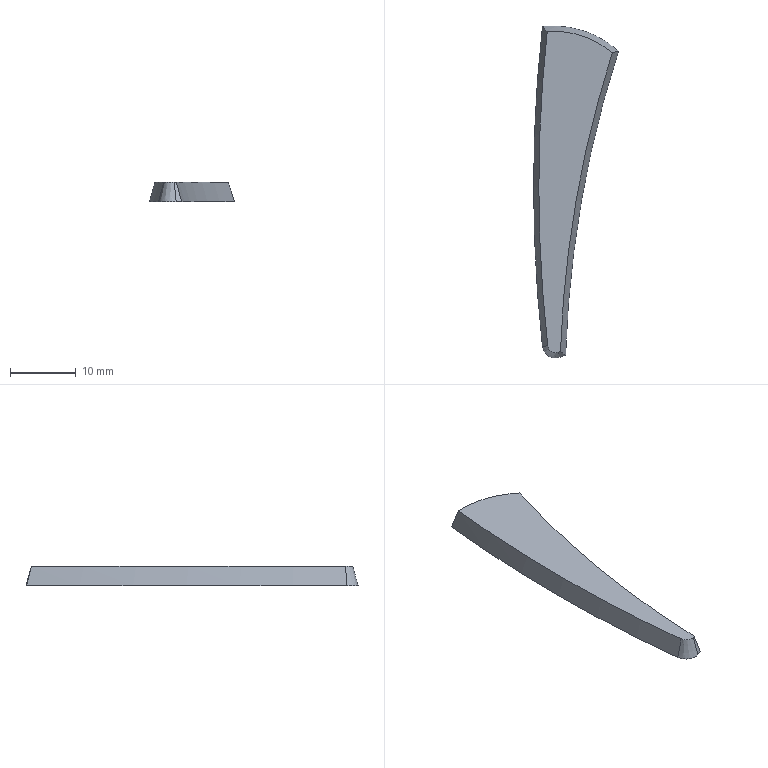Part | STEP file | Twistgrip Indicator LensMirror 3 speed | 1 solid | 7 faces | box 12.929 x 50.6 x 3 mm | volume 990.218 mm3 | cone 4 | plane 3
STEP:
#1=CARTESIAN_POINT('',(0.,0.,0.));
#2=DIRECTION('',(0.,0.,1.));
#3=DIRECTION('',(1.,0.,0.));
#4=AXIS2_PLACEMENT_3D('',#1,#2,#3);
#5=CARTESIAN_POINT('',(-17.743,-15.241,-3.));
#6=VERTEX_POINT('',#5);
#7=CARTESIAN_POINT('',(-18.67,-15.499,0.));
#8=VERTEX_POINT('',#7);
#9=CARTESIAN_POINT('',(-17.743,-15.241,-3.));
#10=CARTESIAN_POINT('',(-18.051,-15.323,-1.999));
#11=CARTESIAN_POINT('',(-18.36,-15.409,-0.9995));
#12=CARTESIAN_POINT('',(-18.67,-15.499,0.));
#13=B_SPLINE_CURVE_WITH_KNOTS('',3,(#9,#10,#11,#12),.UNSPECIFIED.,.F.,.F.,(4,4),(0.,0.003151),.PIECEWISE_BEZIER_KNOTS.);
#14=CARTESIAN_POINT('',(142.328,-66.926,0.));
#15=DIRECTION('',(0.,0.,1.));
#16=DIRECTION('',(1.,0.,0.));
#17=AXIS2_PLACEMENT_3D('',#14,#15,#16);
#18=CONICAL_SURFACE('',#17,169.012,0.2618);
#19=CARTESIAN_POINT('',(2.829,-3.));
#20=CARTESIAN_POINT('',(2.829,-2.955));
#21=CARTESIAN_POINT('',(2.829,-2.864));
#22=CARTESIAN_POINT('',(2.83,-2.727));
#23=CARTESIAN_POINT('',(2.83,-2.591));
#24=CARTESIAN_POINT('',(2.83,-2.454));
#25=CARTESIAN_POINT('',(2.83,-2.318));
#26=CARTESIAN_POINT('',(2.83,-2.182));
#27=CARTESIAN_POINT('',(2.83,-2.045));
#28=CARTESIAN_POINT('',(2.83,-1.909));
#29=CARTESIAN_POINT('',(2.831,-1.772));
#30=CARTESIAN_POINT('',(2.831,-1.636));
#31=CARTESIAN_POINT('',(2.831,-1.5));
#32=CARTESIAN_POINT('',(2.831,-1.363));
#33=CARTESIAN_POINT('',(2.831,-1.227));
#34=CARTESIAN_POINT('',(2.831,-1.091));
#35=CARTESIAN_POINT('',(2.831,-0.9542));
#36=CARTESIAN_POINT('',(2.832,-0.8179));
#37=CARTESIAN_POINT('',(2.832,-0.6815));
#38=CARTESIAN_POINT('',(2.832,-0.5452));
#39=CARTESIAN_POINT('',(2.832,-0.4089));
#40=CARTESIAN_POINT('',(2.832,-0.2726));
#41=CARTESIAN_POINT('',(2.832,-0.1363));
#42=CARTESIAN_POINT('',(2.832,-0.04543));
#43=CARTESIAN_POINT('',(2.832,0.));
#44=B_SPLINE_CURVE_WITH_KNOTS('',3,(#19,#20,#21,#22,#23,#24,#25,#26,#27,#28,#29,#30,#31,#32,#33,#34,#35,#36,#37,#38,#39,#40,#41,#42,#43),.UNSPECIFIED.,.F.,.F.,(4,1,1,1,1,1,1,1,1,1,1,1,1,1,1,1,1,1,1,1,1,1,4),(0.,0.0001432,0.0002864,0.0004296,0.0005728,0.000716,0.0008592,0.001002,0.001146,0.001289,0.001432,0.001575,0.001718,0.001862,0.002005,0.002148,0.002291,0.002435,0.002578,0.002721,0.002864,0.003007,0.003151),.QUASI_UNIFORM_KNOTS.);
#45=(GEOMETRIC_REPRESENTATION_CONTEXT(2)PARAMETRIC_REPRESENTATION_CONTEXT()REPRESENTATION_CONTEXT('',''));
#46=DEFINITIONAL_REPRESENTATION('',(#44),#45);
#47=PCURVE('',#18,#46);
#48=CARTESIAN_POINT('',(-27.685,-26.228,0.));
#49=DIRECTION('',(0.,0.,-1.));
#50=DIRECTION('',(1.,0.,0.));
#51=AXIS2_PLACEMENT_3D('',#48,#49,#50);
#52=CONICAL_SURFACE('',#51,14.014,0.2618);
#53=CARTESIAN_POINT('',(5.448,3.));
#54=CARTESIAN_POINT('',(5.447,2.955));
#55=CARTESIAN_POINT('',(5.446,2.864));
#56=CARTESIAN_POINT('',(5.445,2.727));
#57=CARTESIAN_POINT('',(5.443,2.591));
#58=CARTESIAN_POINT('',(5.441,2.454));
#59=CARTESIAN_POINT('',(5.44,2.318));
#60=CARTESIAN_POINT('',(5.438,2.182));
#61=CARTESIAN_POINT('',(5.437,2.045));
#62=CARTESIAN_POINT('',(5.435,1.909));
#63=CARTESIAN_POINT('',(5.433,1.772));
#64=CARTESIAN_POINT('',(5.432,1.636));
#65=CARTESIAN_POINT('',(5.43,1.5));
#66=CARTESIAN_POINT('',(5.428,1.363));
#67=CARTESIAN_POINT('',(5.427,1.227));
#68=CARTESIAN_POINT('',(5.425,1.091));
#69=CARTESIAN_POINT('',(5.423,0.9542));
#70=CARTESIAN_POINT('',(5.422,0.8179));
#71=CARTESIAN_POINT('',(5.42,0.6815));
#72=CARTESIAN_POINT('',(5.418,0.5452));
#73=CARTESIAN_POINT('',(5.416,0.4089));
#74=CARTESIAN_POINT('',(5.415,0.2726));
#75=CARTESIAN_POINT('',(5.413,0.1363));
#76=CARTESIAN_POINT('',(5.412,0.04543));
#77=CARTESIAN_POINT('',(5.411,0.));
#78=B_SPLINE_CURVE_WITH_KNOTS('',3,(#53,#54,#55,#56,#57,#58,#59,#60,#61,#62,#63,#64,#65,#66,#67,#68,#69,#70,#71,#72,#73,#74,#75,#76,#77),.UNSPECIFIED.,.F.,.F.,(4,1,1,1,1,1,1,1,1,1,1,1,1,1,1,1,1,1,1,1,1,1,4),(0.,0.0001432,0.0002864,0.0004296,0.0005728,0.000716,0.0008592,0.001002,0.001146,0.001289,0.001432,0.001575,0.001718,0.001862,0.002005,0.002148,0.002291,0.002435,0.002578,0.002721,0.002864,0.003007,0.003151),.QUASI_UNIFORM_KNOTS.);
#79=(GEOMETRIC_REPRESENTATION_CONTEXT(2)PARAMETRIC_REPRESENTATION_CONTEXT()REPRESENTATION_CONTEXT('',''));
#80=DEFINITIONAL_REPRESENTATION('',(#78),#79);
#81=PCURVE('',#52,#80);
#82=SURFACE_CURVE('',#13,(#47,#81),.PCURVE_S1.);
#83=EDGE_CURVE('',#6,#8,#82,.T.);
#84=ORIENTED_EDGE('',*,*,#83,.F.);
#85=CARTESIAN_POINT('',(-25.795,-61.568,-3.));
#86=VERTEX_POINT('',#85);
#87=CARTESIAN_POINT('',(142.328,-66.926,-3.));
#88=DIRECTION('',(0.,0.,-1.));
#89=DIRECTION('',(1.,0.,0.));
#90=AXIS2_PLACEMENT_3D('',#87,#88,#89);
#91=CIRCLE('',#90,168.208);
#92=CARTESIAN_POINT('',(6.283,-3.));
#93=DIRECTION('',(-1.,0.));
#94=VECTOR('',#93,1.);
#95=LINE('',#92,#94);
#96=(GEOMETRIC_REPRESENTATION_CONTEXT(2)PARAMETRIC_REPRESENTATION_CONTEXT()REPRESENTATION_CONTEXT('',''));
#97=DEFINITIONAL_REPRESENTATION('',(#95),#96);
#98=PCURVE('',#18,#97);
#99=CARTESIAN_POINT('',(142.328,-66.926,-3.));
#100=DIRECTION('',(0.,0.,-1.));
#101=DIRECTION('',(1.,0.,0.));
#102=AXIS2_PLACEMENT_3D('',#99,#100,#101);
#103=PLANE('',#102);
#104=CARTESIAN_POINT('',(0.,0.));
#105=DIRECTION('',(1.,0.));
#106=AXIS2_PLACEMENT_2D('',#104,#105);
#107=CIRCLE('',#106,168.208);
#108=(GEOMETRIC_REPRESENTATION_CONTEXT(2)PARAMETRIC_REPRESENTATION_CONTEXT()REPRESENTATION_CONTEXT('',''));
#109=DEFINITIONAL_REPRESENTATION('',(#107),#108);
#110=PCURVE('',#103,#109);
#111=SURFACE_CURVE('',#91,(#98,#110),.PCURVE_S1.);
#112=EDGE_CURVE('',#86,#6,#111,.T.);
#113=ORIENTED_EDGE('',*,*,#112,.F.);
#114=CARTESIAN_POINT('',(-26.58,-61.005,0.));
#115=VERTEX_POINT('',#114);
#116=CARTESIAN_POINT('',(-25.795,-61.568,-3.));
#117=CARTESIAN_POINT('',(-26.057,-61.381,-2.));
#118=CARTESIAN_POINT('',(-26.319,-61.193,-1.));
#119=CARTESIAN_POINT('',(-26.58,-61.005,0.));
#120=B_SPLINE_CURVE_WITH_KNOTS('',3,(#116,#117,#118,#119),.UNSPECIFIED.,.F.,.F.,(4,4),(0.,0.003152),.PIECEWISE_BEZIER_KNOTS.);
#121=CARTESIAN_POINT('',(3.11,-3.));
#122=CARTESIAN_POINT('',(3.11,-2.955));
#123=CARTESIAN_POINT('',(3.11,-2.864));
#124=CARTESIAN_POINT('',(3.109,-2.727));
#125=CARTESIAN_POINT('',(3.109,-2.591));
#126=CARTESIAN_POINT('',(3.109,-2.455));
#127=CARTESIAN_POINT('',(3.109,-2.318));
#128=CARTESIAN_POINT('',(3.109,-2.182));
#129=CARTESIAN_POINT('',(3.109,-2.045));
#130=CARTESIAN_POINT('',(3.109,-1.909));
#131=CARTESIAN_POINT('',(3.108,-1.773));
#132=CARTESIAN_POINT('',(3.108,-1.636));
#133=CARTESIAN_POINT('',(3.108,-1.5));
#134=CARTESIAN_POINT('',(3.108,-1.364));
#135=CARTESIAN_POINT('',(3.108,-1.227));
#136=CARTESIAN_POINT('',(3.108,-1.091));
#137=CARTESIAN_POINT('',(3.108,-0.9546));
#138=CARTESIAN_POINT('',(3.107,-0.8182));
#139=CARTESIAN_POINT('',(3.107,-0.6818));
#140=CARTESIAN_POINT('',(3.107,-0.5455));
#141=CARTESIAN_POINT('',(3.107,-0.4091));
#142=CARTESIAN_POINT('',(3.107,-0.2727));
#143=CARTESIAN_POINT('',(3.107,-0.1364));
#144=CARTESIAN_POINT('',(3.107,-0.04546));
#145=CARTESIAN_POINT('',(3.107,0.));
#146=B_SPLINE_CURVE_WITH_KNOTS('',3,(#121,#122,#123,#124,#125,#126,#127,#128,#129,#130,#131,#132,#133,#134,#135,#136,#137,#138,#139,#140,#141,#142,#143,#144,#145),.UNSPECIFIED.,.F.,.F.,(4,1,1,1,1,1,1,1,1,1,1,1,1,1,1,1,1,1,1,1,1,1,4),(0.,0.0001433,0.0002865,0.0004298,0.0005731,0.0007163,0.0008596,0.001003,0.001146,0.001289,0.001433,0.001576,0.001719,0.001862,0.002006,0.002149,0.002292,0.002435,0.002579,0.002722,0.002865,0.003009,0.003152),.QUASI_UNIFORM_KNOTS.);
#147=(GEOMETRIC_REPRESENTATION_CONTEXT(2)PARAMETRIC_REPRESENTATION_CONTEXT()REPRESENTATION_CONTEXT('',''));
#148=DEFINITIONAL_REPRESENTATION('',(#146),#147);
#149=PCURVE('',#18,#148);
#150=CARTESIAN_POINT('',(-26.909,-61.129,0.));
#151=DIRECTION('',(0.3409,-0.9038,0.2588));
#152=DIRECTION('',(0.9357,0.3529,0.));
#153=AXIS2_PLACEMENT_3D('',#150,#151,#152);
#154=PLANE('',#153);
#155=CARTESIAN_POINT('',(0.8877,-3.106));
#156=CARTESIAN_POINT('',(0.7086,-2.071));
#157=CARTESIAN_POINT('',(0.5298,-1.035));
#158=CARTESIAN_POINT('',(0.3514,0.));
#159=B_SPLINE_CURVE_WITH_KNOTS('',3,(#155,#156,#157,#158),.UNSPECIFIED.,.F.,.F.,(4,4),(0.,0.003152),.PIECEWISE_BEZIER_KNOTS.);
#160=(GEOMETRIC_REPRESENTATION_CONTEXT(2)PARAMETRIC_REPRESENTATION_CONTEXT()REPRESENTATION_CONTEXT('',''));
#161=DEFINITIONAL_REPRESENTATION('',(#159),#160);
#162=PCURVE('',#154,#161);
#163=SURFACE_CURVE('',#120,(#149,#162),.PCURVE_S1.);
#164=EDGE_CURVE('',#86,#115,#163,.T.);
#165=ORIENTED_EDGE('',*,*,#164,.T.);
#166=CARTESIAN_POINT('',(142.328,-66.926,0.));
#167=DIRECTION('',(0.,0.,-1.));
#168=DIRECTION('',(1.,0.,0.));
#169=AXIS2_PLACEMENT_3D('',#166,#167,#168);
#170=CIRCLE('',#169,169.012);
#171=CARTESIAN_POINT('',(6.283,0.));
#172=DIRECTION('',(-1.,0.));
#173=VECTOR('',#172,1.);
#174=LINE('',#171,#173);
#175=(GEOMETRIC_REPRESENTATION_CONTEXT(2)PARAMETRIC_REPRESENTATION_CONTEXT()REPRESENTATION_CONTEXT('',''));
#176=DEFINITIONAL_REPRESENTATION('',(#174),#175);
#177=PCURVE('',#18,#176);
#178=CARTESIAN_POINT('',(142.328,-66.926,0.));
#179=DIRECTION('',(0.,0.,-1.));
#180=DIRECTION('',(1.,0.,0.));
#181=AXIS2_PLACEMENT_3D('',#178,#179,#180);
#182=PLANE('',#181);
#183=CARTESIAN_POINT('',(0.,0.));
#184=DIRECTION('',(1.,0.));
#185=AXIS2_PLACEMENT_2D('',#183,#184);
#186=CIRCLE('',#185,169.012);
#187=(GEOMETRIC_REPRESENTATION_CONTEXT(2)PARAMETRIC_REPRESENTATION_CONTEXT()REPRESENTATION_CONTEXT('',''));
#188=DEFINITIONAL_REPRESENTATION('',(#186),#187);
#189=PCURVE('',#182,#188);
#190=SURFACE_CURVE('',#170,(#177,#189),.PCURVE_S1.);
#191=EDGE_CURVE('',#115,#8,#190,.T.);
#192=ORIENTED_EDGE('',*,*,#191,.T.);
#193=EDGE_LOOP('',(#84,#113,#165,#192));
#194=FACE_BOUND('',#193,.F.);
#195=ADVANCED_FACE('',(#194),#18,.F.);
#196=CARTESIAN_POINT('',(-28.597,-12.244,0.));
#197=VERTEX_POINT('',#196);
#198=CARTESIAN_POINT('',(-27.685,-26.228,0.));
#199=DIRECTION('',(0.,0.,1.));
#200=DIRECTION('',(1.,0.,0.));
#201=AXIS2_PLACEMENT_3D('',#198,#199,#200);
#202=CIRCLE('',#201,14.014);
#203=CARTESIAN_POINT('',(6.283,0.));
#204=DIRECTION('',(-1.,0.));
#205=VECTOR('',#204,1.);
#206=LINE('',#203,#205);
#207=(GEOMETRIC_REPRESENTATION_CONTEXT(2)PARAMETRIC_REPRESENTATION_CONTEXT()REPRESENTATION_CONTEXT('',''));
#208=DEFINITIONAL_REPRESENTATION('',(#206),#207);
#209=PCURVE('',#52,#208);
#210=CARTESIAN_POINT('',(-155.999,-40.698));
#211=CARTESIAN_POINT('',(-155.999,-64.971));
#212=CARTESIAN_POINT('',(-177.02,-52.835));
#213=CARTESIAN_POINT('',(-198.041,-40.698));
#214=CARTESIAN_POINT('',(-177.02,-28.561));
#215=CARTESIAN_POINT('',(-155.999,-16.425));
#216=CARTESIAN_POINT('',(-155.999,-40.698));
#217=(BOUNDED_CURVE()B_SPLINE_CURVE(2,(#210,#211,#212,#213,#214,#215,#216),.UNSPECIFIED.,.T.,.F.)B_SPLINE_CURVE_WITH_KNOTS((1,2,2,2,2,1),(-2.094,0.,2.094,4.189,6.283,8.378),.UNSPECIFIED.)CURVE()GEOMETRIC_REPRESENTATION_ITEM()RATIONAL_B_SPLINE_CURVE((1.,0.5,1.,0.5,1.,0.5,1.))REPRESENTATION_ITEM(''));
#218=(GEOMETRIC_REPRESENTATION_CONTEXT(2)PARAMETRIC_REPRESENTATION_CONTEXT()REPRESENTATION_CONTEXT('',''));
#219=DEFINITIONAL_REPRESENTATION('',(#217),#218);
#220=PCURVE('',#182,#219);
#221=SURFACE_CURVE('',#202,(#209,#220),.PCURVE_S1.);
#222=EDGE_CURVE('',#8,#197,#221,.T.);
#223=ORIENTED_EDGE('',*,*,#222,.F.);
#224=ORIENTED_EDGE('',*,*,#83,.F.);
#225=CARTESIAN_POINT('',(-29.325,-11.501,-3.));
#226=VERTEX_POINT('',#225);
#227=CARTESIAN_POINT('',(-27.685,-26.228,-3.));
#228=DIRECTION('',(0.,0.,1.));
#229=DIRECTION('',(1.,0.,0.));
#230=AXIS2_PLACEMENT_3D('',#227,#228,#229);
#231=CIRCLE('',#230,14.818);
#232=CARTESIAN_POINT('',(6.283,3.));
#233=DIRECTION('',(-1.,0.));
#234=VECTOR('',#233,1.);
#235=LINE('',#232,#234);
#236=(GEOMETRIC_REPRESENTATION_CONTEXT(2)PARAMETRIC_REPRESENTATION_CONTEXT()REPRESENTATION_CONTEXT('',''));
#237=DEFINITIONAL_REPRESENTATION('',(#235),#236);
#238=PCURVE('',#52,#237);
#239=CARTESIAN_POINT('',(-155.195,-40.698));
#240=CARTESIAN_POINT('',(-155.195,-66.364));
#241=CARTESIAN_POINT('',(-177.422,-53.531));
#242=CARTESIAN_POINT('',(-199.649,-40.698));
#243=CARTESIAN_POINT('',(-177.422,-27.865));
#244=CARTESIAN_POINT('',(-155.195,-15.032));
#245=CARTESIAN_POINT('',(-155.195,-40.698));
#246=(BOUNDED_CURVE()B_SPLINE_CURVE(2,(#239,#240,#241,#242,#243,#244,#245),.UNSPECIFIED.,.T.,.F.)B_SPLINE_CURVE_WITH_KNOTS((1,2,2,2,2,1),(-2.094,0.,2.094,4.189,6.283,8.378),.UNSPECIFIED.)CURVE()GEOMETRIC_REPRESENTATION_ITEM()RATIONAL_B_SPLINE_CURVE((1.,0.5,1.,0.5,1.,0.5,1.))REPRESENTATION_ITEM(''));
#247=(GEOMETRIC_REPRESENTATION_CONTEXT(2)PARAMETRIC_REPRESENTATION_CONTEXT()REPRESENTATION_CONTEXT('',''));
#248=DEFINITIONAL_REPRESENTATION('',(#246),#247);
#249=PCURVE('',#103,#248);
#250=SURFACE_CURVE('',#231,(#238,#249),.PCURVE_S1.);
#251=EDGE_CURVE('',#6,#226,#250,.T.);
#252=ORIENTED_EDGE('',*,*,#251,.T.);
#253=CARTESIAN_POINT('',(-29.325,-11.501,-3.));
#254=CARTESIAN_POINT('',(-29.082,-11.744,-1.999));
#255=CARTESIAN_POINT('',(-28.839,-11.991,-0.9989));
#256=CARTESIAN_POINT('',(-28.597,-12.244,0.));
#257=B_SPLINE_CURVE_WITH_KNOTS('',3,(#253,#254,#255,#256),.UNSPECIFIED.,.F.,.F.,(4,4),(0.,0.003175),.PIECEWISE_BEZIER_KNOTS.);
#258=CARTESIAN_POINT('',(4.602,3.));
#259=CARTESIAN_POINT('',(4.602,2.954));
#260=CARTESIAN_POINT('',(4.603,2.863));
#261=CARTESIAN_POINT('',(4.605,2.727));
#262=CARTESIAN_POINT('',(4.607,2.591));
#263=CARTESIAN_POINT('',(4.609,2.454));
#264=CARTESIAN_POINT('',(4.612,2.318));
#265=CARTESIAN_POINT('',(4.614,2.181));
#266=CARTESIAN_POINT('',(4.616,2.045));
#267=CARTESIAN_POINT('',(4.618,1.908));
#268=CARTESIAN_POINT('',(4.62,1.772));
#269=CARTESIAN_POINT('',(4.622,1.636));
#270=CARTESIAN_POINT('',(4.624,1.499));
#271=CARTESIAN_POINT('',(4.626,1.363));
#272=CARTESIAN_POINT('',(4.628,1.226));
#273=CARTESIAN_POINT('',(4.63,1.09));
#274=CARTESIAN_POINT('',(4.632,0.9538));
#275=CARTESIAN_POINT('',(4.634,0.8175));
#276=CARTESIAN_POINT('',(4.636,0.6812));
#277=CARTESIAN_POINT('',(4.639,0.545));
#278=CARTESIAN_POINT('',(4.641,0.4087));
#279=CARTESIAN_POINT('',(4.643,0.2725));
#280=CARTESIAN_POINT('',(4.645,0.1362));
#281=CARTESIAN_POINT('',(4.647,0.0454));
#282=CARTESIAN_POINT('',(4.647,0.));
#283=B_SPLINE_CURVE_WITH_KNOTS('',3,(#258,#259,#260,#261,#262,#263,#264,#265,#266,#267,#268,#269,#270,#271,#272,#273,#274,#275,#276,#277,#278,#279,#280,#281,#282),.UNSPECIFIED.,.F.,.F.,(4,1,1,1,1,1,1,1,1,1,1,1,1,1,1,1,1,1,1,1,1,1,4),(0.,0.0001443,0.0002886,0.000433,0.0005773,0.0007216,0.0008659,0.00101,0.001155,0.001299,0.001443,0.001587,0.001732,0.001876,0.00202,0.002165,0.002309,0.002453,0.002598,0.002742,0.002886,0.003031,0.003175),.QUASI_UNIFORM_KNOTS.);
#284=(GEOMETRIC_REPRESENTATION_CONTEXT(2)PARAMETRIC_REPRESENTATION_CONTEXT()REPRESENTATION_CONTEXT('',''));
#285=DEFINITIONAL_REPRESENTATION('',(#283),#284);
#286=PCURVE('',#52,#285);
#287=CARTESIAN_POINT('',(189.878,-35.84,0.));
#288=DIRECTION('',(0.,0.,-1.));
#289=DIRECTION('',(1.,0.,0.));
#290=AXIS2_PLACEMENT_3D('',#287,#288,#289);
#291=CONICAL_SURFACE('',#290,219.746,0.2618);
#292=CARTESIAN_POINT('',(3.252,3.));
#293=CARTESIAN_POINT('',(3.252,2.954));
#294=CARTESIAN_POINT('',(3.252,2.863));
#295=CARTESIAN_POINT('',(3.252,2.727));
#296=CARTESIAN_POINT('',(3.252,2.591));
#297=CARTESIAN_POINT('',(3.252,2.454));
#298=CARTESIAN_POINT('',(3.252,2.318));
#299=CARTESIAN_POINT('',(3.251,2.181));
#300=CARTESIAN_POINT('',(3.251,2.045));
#301=CARTESIAN_POINT('',(3.251,1.908));
#302=CARTESIAN_POINT('',(3.251,1.772));
#303=CARTESIAN_POINT('',(3.251,1.636));
#304=CARTESIAN_POINT('',(3.251,1.499));
#305=CARTESIAN_POINT('',(3.251,1.363));
#306=CARTESIAN_POINT('',(3.25,1.226));
#307=CARTESIAN_POINT('',(3.25,1.09));
#308=CARTESIAN_POINT('',(3.25,0.9538));
#309=CARTESIAN_POINT('',(3.25,0.8175));
#310=CARTESIAN_POINT('',(3.25,0.6812));
#311=CARTESIAN_POINT('',(3.25,0.545));
#312=CARTESIAN_POINT('',(3.25,0.4087));
#313=CARTESIAN_POINT('',(3.249,0.2725));
#314=CARTESIAN_POINT('',(3.249,0.1362));
#315=CARTESIAN_POINT('',(3.249,0.0454));
#316=CARTESIAN_POINT('',(3.249,0.));
#317=B_SPLINE_CURVE_WITH_KNOTS('',3,(#292,#293,#294,#295,#296,#297,#298,#299,#300,#301,#302,#303,#304,#305,#306,#307,#308,#309,#310,#311,#312,#313,#314,#315,#316),.UNSPECIFIED.,.F.,.F.,(4,1,1,1,1,1,1,1,1,1,1,1,1,1,1,1,1,1,1,1,1,1,4),(0.,0.0001443,0.0002886,0.000433,0.0005773,0.0007216,0.0008659,0.00101,0.001155,0.001299,0.001443,0.001587,0.001732,0.001876,0.00202,0.002165,0.002309,0.002453,0.002598,0.002742,0.002886,0.003031,0.003175),.QUASI_UNIFORM_KNOTS.);
#318=(GEOMETRIC_REPRESENTATION_CONTEXT(2)PARAMETRIC_REPRESENTATION_CONTEXT()REPRESENTATION_CONTEXT('',''));
#319=DEFINITIONAL_REPRESENTATION('',(#317),#318);
#320=PCURVE('',#291,#319);
#321=SURFACE_CURVE('',#257,(#286,#320),.PCURVE_S1.);
#322=EDGE_CURVE('',#226,#197,#321,.T.);
#323=ORIENTED_EDGE('',*,*,#322,.T.);
#324=EDGE_LOOP('',(#223,#224,#252,#323));
#325=FACE_BOUND('',#324,.T.);
#326=ADVANCED_FACE('',(#325),#52,.T.);
#327=CARTESIAN_POINT('',(-28.52,-60.142,0.));
#328=VERTEX_POINT('',#327);
#329=CARTESIAN_POINT('',(189.878,-35.84,0.));
#330=DIRECTION('',(0.,0.,1.));
#331=DIRECTION('',(1.,0.,0.));
#332=AXIS2_PLACEMENT_3D('',#329,#330,#331);
#333=CIRCLE('',#332,219.746);
#334=CARTESIAN_POINT('',(6.283,0.));
#335=DIRECTION('',(-1.,0.));
#336=VECTOR('',#335,1.);
#337=LINE('',#334,#336);
#338=(GEOMETRIC_REPRESENTATION_CONTEXT(2)PARAMETRIC_REPRESENTATION_CONTEXT()REPRESENTATION_CONTEXT('',''));
#339=DEFINITIONAL_REPRESENTATION('',(#337),#338);
#340=PCURVE('',#291,#339);
#341=CARTESIAN_POINT('',(267.297,-31.086));
#342=CARTESIAN_POINT('',(267.297,-411.698));
#343=CARTESIAN_POINT('',(-62.323,-221.392));
#344=CARTESIAN_POINT('',(-391.942,-31.086));
#345=CARTESIAN_POINT('',(-62.323,159.22));
#346=CARTESIAN_POINT('',(267.297,349.526));
#347=CARTESIAN_POINT('',(267.297,-31.086));
#348=(BOUNDED_CURVE()B_SPLINE_CURVE(2,(#341,#342,#343,#344,#345,#346,#347),.UNSPECIFIED.,.T.,.F.)B_SPLINE_CURVE_WITH_KNOTS((1,2,2,2,2,1),(-2.094,0.,2.094,4.189,6.283,8.378),.UNSPECIFIED.)CURVE()GEOMETRIC_REPRESENTATION_ITEM()RATIONAL_B_SPLINE_CURVE((1.,0.5,1.,0.5,1.,0.5,1.))REPRESENTATION_ITEM(''));
#349=(GEOMETRIC_REPRESENTATION_CONTEXT(2)PARAMETRIC_REPRESENTATION_CONTEXT()REPRESENTATION_CONTEXT('',''));
#350=DEFINITIONAL_REPRESENTATION('',(#348),#349);
#351=PCURVE('',#182,#350);
#352=SURFACE_CURVE('',#333,(#340,#351),.PCURVE_S1.);
#353=EDGE_CURVE('',#197,#328,#352,.T.);
#354=ORIENTED_EDGE('',*,*,#353,.F.);
#355=ORIENTED_EDGE('',*,*,#322,.F.);
#356=CARTESIAN_POINT('',(-29.319,-60.231,-3.));
#357=VERTEX_POINT('',#356);
#358=CARTESIAN_POINT('',(189.878,-35.84,-3.));
#359=DIRECTION('',(0.,0.,1.));
#360=DIRECTION('',(1.,0.,0.));
#361=AXIS2_PLACEMENT_3D('',#358,#359,#360);
#362=CIRCLE('',#361,220.55);
#363=CARTESIAN_POINT('',(6.283,3.));
#364=DIRECTION('',(-1.,0.));
#365=VECTOR('',#364,1.);
#366=LINE('',#363,#365);
#367=(GEOMETRIC_REPRESENTATION_CONTEXT(2)PARAMETRIC_REPRESENTATION_CONTEXT()REPRESENTATION_CONTEXT('',''));
#368=DEFINITIONAL_REPRESENTATION('',(#366),#367);
#369=PCURVE('',#291,#368);
#370=CARTESIAN_POINT('',(268.101,-31.086));
#371=CARTESIAN_POINT('',(268.101,-413.09));
#372=CARTESIAN_POINT('',(-62.724,-222.088));
#373=CARTESIAN_POINT('',(-393.55,-31.086));
#374=CARTESIAN_POINT('',(-62.724,159.916));
#375=CARTESIAN_POINT('',(268.101,350.918));
#376=CARTESIAN_POINT('',(268.101,-31.086));
#377=(BOUNDED_CURVE()B_SPLINE_CURVE(2,(#370,#371,#372,#373,#374,#375,#376),.UNSPECIFIED.,.T.,.F.)B_SPLINE_CURVE_WITH_KNOTS((1,2,2,2,2,1),(-2.094,0.,2.094,4.189,6.283,8.378),.UNSPECIFIED.)CURVE()GEOMETRIC_REPRESENTATION_ITEM()RATIONAL_B_SPLINE_CURVE((1.,0.5,1.,0.5,1.,0.5,1.))REPRESENTATION_ITEM(''));
#378=(GEOMETRIC_REPRESENTATION_CONTEXT(2)PARAMETRIC_REPRESENTATION_CONTEXT()REPRESENTATION_CONTEXT('',''));
#379=DEFINITIONAL_REPRESENTATION('',(#377),#378);
#380=PCURVE('',#103,#379);
#381=SURFACE_CURVE('',#362,(#369,#380),.PCURVE_S1.);
#382=EDGE_CURVE('',#226,#357,#381,.T.);
#383=ORIENTED_EDGE('',*,*,#382,.T.);
#384=CARTESIAN_POINT('',(-28.52,-60.142,0.));
#385=DIRECTION('',(0.2572,0.02862,0.9659));
#386=VECTOR('',#385,1.);
#387=LINE('',#384,#386);
#388=CARTESIAN_POINT('',(3.031,0.));
#389=DIRECTION('',(0.,-1.));
#390=VECTOR('',#389,1.);
#391=LINE('',#388,#390);
#392=(GEOMETRIC_REPRESENTATION_CONTEXT(2)PARAMETRIC_REPRESENTATION_CONTEXT()REPRESENTATION_CONTEXT('',''));
#393=DEFINITIONAL_REPRESENTATION('',(#391),#392);
#394=PCURVE('',#291,#393);
#395=CARTESIAN_POINT('',(-27.331,-60.01,0.));
#396=DIRECTION('',(0.,0.,-1.));
#397=DIRECTION('',(1.,0.,0.));
#398=AXIS2_PLACEMENT_3D('',#395,#396,#397);
#399=CONICAL_SURFACE('',#398,1.196,0.2618);
#400=CARTESIAN_POINT('',(3.031,0.));
#401=DIRECTION('',(0.,-1.));
#402=VECTOR('',#401,1.);
#403=LINE('',#400,#402);
#404=(GEOMETRIC_REPRESENTATION_CONTEXT(2)PARAMETRIC_REPRESENTATION_CONTEXT()REPRESENTATION_CONTEXT('',''));
#405=DEFINITIONAL_REPRESENTATION('',(#403),#404);
#406=PCURVE('',#399,#405);
#407=SURFACE_CURVE('',#387,(#394,#406),.PCURVE_S1.);
#408=EDGE_CURVE('',#357,#328,#407,.T.);
#409=ORIENTED_EDGE('',*,*,#408,.T.);
#410=EDGE_LOOP('',(#354,#355,#383,#409));
#411=FACE_BOUND('',#410,.T.);
#412=ADVANCED_FACE('',(#411),#291,.T.);
#413=CARTESIAN_POINT('',(-26.909,-61.129,0.));
#414=VERTEX_POINT('',#413);
#415=CARTESIAN_POINT('',(-27.331,-60.01,0.));
#416=DIRECTION('',(0.,0.,1.));
#417=DIRECTION('',(1.,0.,0.));
#418=AXIS2_PLACEMENT_3D('',#415,#416,#417);
#419=CIRCLE('',#418,1.196);
#420=CARTESIAN_POINT('',(6.283,0.));
#421=DIRECTION('',(-1.,0.));
#422=VECTOR('',#421,1.);
#423=LINE('',#420,#422);
#424=(GEOMETRIC_REPRESENTATION_CONTEXT(2)PARAMETRIC_REPRESENTATION_CONTEXT()REPRESENTATION_CONTEXT('',''));
#425=DEFINITIONAL_REPRESENTATION('',(#423),#424);
#426=PCURVE('',#399,#425);
#427=CARTESIAN_POINT('',(-168.463,-6.916));
#428=CARTESIAN_POINT('',(-168.463,-8.988));
#429=CARTESIAN_POINT('',(-170.257,-7.952));
#430=CARTESIAN_POINT('',(-172.051,-6.916));
#431=CARTESIAN_POINT('',(-170.257,-5.88));
#432=CARTESIAN_POINT('',(-168.463,-4.844));
#433=CARTESIAN_POINT('',(-168.463,-6.916));
#434=(BOUNDED_CURVE()B_SPLINE_CURVE(2,(#427,#428,#429,#430,#431,#432,#433),.UNSPECIFIED.,.T.,.F.)B_SPLINE_CURVE_WITH_KNOTS((1,2,2,2,2,1),(-2.094,0.,2.094,4.189,6.283,8.378),.UNSPECIFIED.)CURVE()GEOMETRIC_REPRESENTATION_ITEM()RATIONAL_B_SPLINE_CURVE((1.,0.5,1.,0.5,1.,0.5,1.))REPRESENTATION_ITEM(''));
#435=(GEOMETRIC_REPRESENTATION_CONTEXT(2)PARAMETRIC_REPRESENTATION_CONTEXT()REPRESENTATION_CONTEXT('',''));
#436=DEFINITIONAL_REPRESENTATION('',(#434),#435);
#437=PCURVE('',#182,#436);
#438=SURFACE_CURVE('',#419,(#426,#437),.PCURVE_S1.);
#439=EDGE_CURVE('',#328,#414,#438,.T.);
#440=ORIENTED_EDGE('',*,*,#439,.F.);
#441=ORIENTED_EDGE('',*,*,#408,.F.);
#442=CARTESIAN_POINT('',(-26.625,-61.881,-3.));
#443=VERTEX_POINT('',#442);
#444=CARTESIAN_POINT('',(-27.331,-60.01,-3.));
#445=DIRECTION('',(0.,0.,1.));
#446=DIRECTION('',(1.,0.,0.));
#447=AXIS2_PLACEMENT_3D('',#444,#445,#446);
#448=CIRCLE('',#447,2.);
#449=CARTESIAN_POINT('',(6.283,3.));
#450=DIRECTION('',(-1.,0.));
#451=VECTOR('',#450,1.);
#452=LINE('',#449,#451);
#453=(GEOMETRIC_REPRESENTATION_CONTEXT(2)PARAMETRIC_REPRESENTATION_CONTEXT()REPRESENTATION_CONTEXT('',''));
#454=DEFINITIONAL_REPRESENTATION('',(#452),#453);
#455=PCURVE('',#399,#454);
#456=CARTESIAN_POINT('',(-167.659,-6.916));
#457=CARTESIAN_POINT('',(-167.659,-10.38));
#458=CARTESIAN_POINT('',(-170.659,-8.648));
#459=CARTESIAN_POINT('',(-173.659,-6.916));
#460=CARTESIAN_POINT('',(-170.659,-5.184));
#461=CARTESIAN_POINT('',(-167.659,-3.452));
#462=CARTESIAN_POINT('',(-167.659,-6.916));
#463=(BOUNDED_CURVE()B_SPLINE_CURVE(2,(#456,#457,#458,#459,#460,#461,#462),.UNSPECIFIED.,.T.,.F.)B_SPLINE_CURVE_WITH_KNOTS((1,2,2,2,2,1),(-2.094,0.,2.094,4.189,6.283,8.378),.UNSPECIFIED.)CURVE()GEOMETRIC_REPRESENTATION_ITEM()RATIONAL_B_SPLINE_CURVE((1.,0.5,1.,0.5,1.,0.5,1.))REPRESENTATION_ITEM(''));
#464=(GEOMETRIC_REPRESENTATION_CONTEXT(2)PARAMETRIC_REPRESENTATION_CONTEXT()REPRESENTATION_CONTEXT('',''));
#465=DEFINITIONAL_REPRESENTATION('',(#463),#464);
#466=PCURVE('',#103,#465);
#467=SURFACE_CURVE('',#448,(#455,#466),.PCURVE_S1.);
#468=EDGE_CURVE('',#357,#443,#467,.T.);
#469=ORIENTED_EDGE('',*,*,#468,.T.);
#470=CARTESIAN_POINT('',(-26.909,-61.129,0.));
#471=DIRECTION('',(-0.09134,0.2422,0.9659));
#472=VECTOR('',#471,1.);
#473=LINE('',#470,#472);
#474=CARTESIAN_POINT('',(1.21,0.));
#475=DIRECTION('',(0.,-1.));
#476=VECTOR('',#475,1.);
#477=LINE('',#474,#476);
#478=(GEOMETRIC_REPRESENTATION_CONTEXT(2)PARAMETRIC_REPRESENTATION_CONTEXT()REPRESENTATION_CONTEXT('',''));
#479=DEFINITIONAL_REPRESENTATION('',(#477),#478);
#480=PCURVE('',#399,#479);
#481=CARTESIAN_POINT('',(0.,0.));
#482=DIRECTION('',(0.,1.));
#483=VECTOR('',#482,1.);
#484=LINE('',#481,#483);
#485=(GEOMETRIC_REPRESENTATION_CONTEXT(2)PARAMETRIC_REPRESENTATION_CONTEXT()REPRESENTATION_CONTEXT('',''));
#486=DEFINITIONAL_REPRESENTATION('',(#484),#485);
#487=PCURVE('',#154,#486);
#488=SURFACE_CURVE('',#473,(#480,#487),.PCURVE_S1.);
#489=EDGE_CURVE('',#443,#414,#488,.T.);
#490=ORIENTED_EDGE('',*,*,#489,.T.);
#491=EDGE_LOOP('',(#440,#441,#469,#490));
#492=FACE_BOUND('',#491,.T.);
#493=ADVANCED_FACE('',(#492),#399,.T.);
#494=CARTESIAN_POINT('',(-26.909,-61.129,0.));
#495=DIRECTION('',(0.9357,0.3529,0.));
#496=VECTOR('',#495,1.);
#497=LINE('',#494,#496);
#498=CARTESIAN_POINT('',(0.,0.));
#499=DIRECTION('',(1.,0.));
#500=VECTOR('',#499,1.);
#501=LINE('',#498,#500);
#502=(GEOMETRIC_REPRESENTATION_CONTEXT(2)PARAMETRIC_REPRESENTATION_CONTEXT()REPRESENTATION_CONTEXT('',''));
#503=DEFINITIONAL_REPRESENTATION('',(#501),#502);
#504=PCURVE('',#154,#503);
#505=CARTESIAN_POINT('',(-169.237,-5.797));
#506=DIRECTION('',(0.9357,-0.3529));
#507=VECTOR('',#506,1.);
#508=LINE('',#505,#507);
#509=(GEOMETRIC_REPRESENTATION_CONTEXT(2)PARAMETRIC_REPRESENTATION_CONTEXT()REPRESENTATION_CONTEXT('',''));
#510=DEFINITIONAL_REPRESENTATION('',(#508),#509);
#511=PCURVE('',#182,#510);
#512=SURFACE_CURVE('',#497,(#504,#511),.PCURVE_S1.);
#513=EDGE_CURVE('',#414,#115,#512,.T.);
#514=ORIENTED_EDGE('',*,*,#513,.F.);
#515=ORIENTED_EDGE('',*,*,#489,.F.);
#516=CARTESIAN_POINT('',(-26.625,-61.881,-3.));
#517=DIRECTION('',(0.9357,0.3529,0.));
#518=VECTOR('',#517,1.);
#519=LINE('',#516,#518);
#520=CARTESIAN_POINT('',(0.,-3.106));
#521=DIRECTION('',(1.,0.));
#522=VECTOR('',#521,1.);
#523=LINE('',#520,#522);
#524=(GEOMETRIC_REPRESENTATION_CONTEXT(2)PARAMETRIC_REPRESENTATION_CONTEXT()REPRESENTATION_CONTEXT('',''));
#525=DEFINITIONAL_REPRESENTATION('',(#523),#524);
#526=PCURVE('',#154,#525);
#527=CARTESIAN_POINT('',(-168.953,-5.045));
#528=DIRECTION('',(0.9357,-0.3529));
#529=VECTOR('',#528,1.);
#530=LINE('',#527,#529);
#531=(GEOMETRIC_REPRESENTATION_CONTEXT(2)PARAMETRIC_REPRESENTATION_CONTEXT()REPRESENTATION_CONTEXT('',''));
#532=DEFINITIONAL_REPRESENTATION('',(#530),#531);
#533=PCURVE('',#103,#532);
#534=SURFACE_CURVE('',#519,(#526,#533),.PCURVE_S1.);
#535=EDGE_CURVE('',#443,#86,#534,.T.);
#536=ORIENTED_EDGE('',*,*,#535,.T.);
#537=ORIENTED_EDGE('',*,*,#164,.T.);
#538=EDGE_LOOP('',(#514,#515,#536,#537));
#539=FACE_BOUND('',#538,.T.);
#540=ADVANCED_FACE('',(#539),#154,.T.);
#541=ORIENTED_EDGE('',*,*,#112,.F.);
#542=ORIENTED_EDGE('',*,*,#535,.F.);
#543=ORIENTED_EDGE('',*,*,#468,.F.);
#544=ORIENTED_EDGE('',*,*,#382,.F.);
#545=ORIENTED_EDGE('',*,*,#251,.F.);
#546=EDGE_LOOP('',(#541,#542,#543,#544,#545));
#547=FACE_BOUND('',#546,.T.);
#548=ADVANCED_FACE('',(#547),#103,.T.);
#549=ORIENTED_EDGE('',*,*,#191,.T.);
#550=ORIENTED_EDGE('',*,*,#222,.T.);
#551=ORIENTED_EDGE('',*,*,#353,.T.);
#552=ORIENTED_EDGE('',*,*,#439,.T.);
#553=ORIENTED_EDGE('',*,*,#513,.T.);
#554=EDGE_LOOP('',(#549,#550,#551,#552,#553));
#555=FACE_BOUND('',#554,.T.);
#556=ADVANCED_FACE('',(#555),#182,.F.);
#557=CLOSED_SHELL('',(#195,#326,#412,#493,#540,#548,#556));
#558=MANIFOLD_SOLID_BREP('',#557);
#559=(LENGTH_UNIT()NAMED_UNIT(*)SI_UNIT(.MILLI.,.METRE.));
#560=UNCERTAINTY_MEASURE_WITH_UNIT(LENGTH_MEASURE(0.0000005),#559,'','');
#561=(NAMED_UNIT(*)PLANE_ANGLE_UNIT()SI_UNIT($,.RADIAN.));
#562=(NAMED_UNIT(*)SI_UNIT($,.STERADIAN.)SOLID_ANGLE_UNIT());
#563=(GEOMETRIC_REPRESENTATION_CONTEXT(3)GLOBAL_UNCERTAINTY_ASSIGNED_CONTEXT((#560))GLOBAL_UNIT_ASSIGNED_CONTEXT((#559,#561,#562))REPRESENTATION_CONTEXT('',''));
#564=ADVANCED_BREP_SHAPE_REPRESENTATION('',(#4,#558),#563);